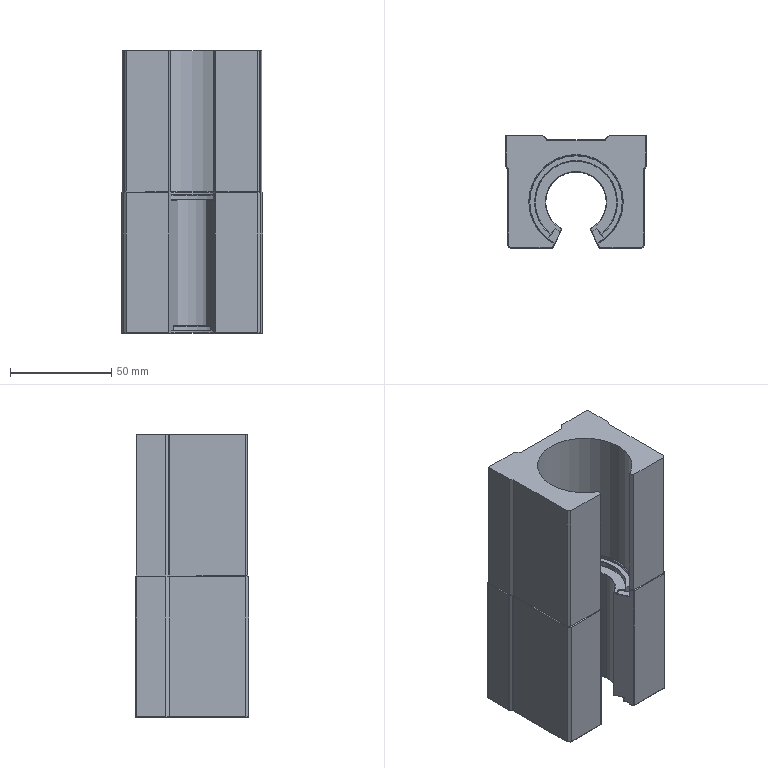Part | SolidWorks | features Fillet 2, ICE 2, RevCut 2, Extrusion 1, SketchPattern 1 | 1 solid | 242 faces | box 70 x 56 x 140 mm | volume 330952 mm3 | cylinder 110 | plane 48 | torus 41 | sphere 26 | spline 17 | commonest cylinder face diameters 0.7 x44 0.35 x34 8 x8 40.73 x6 46.097 x6 1.4 x4